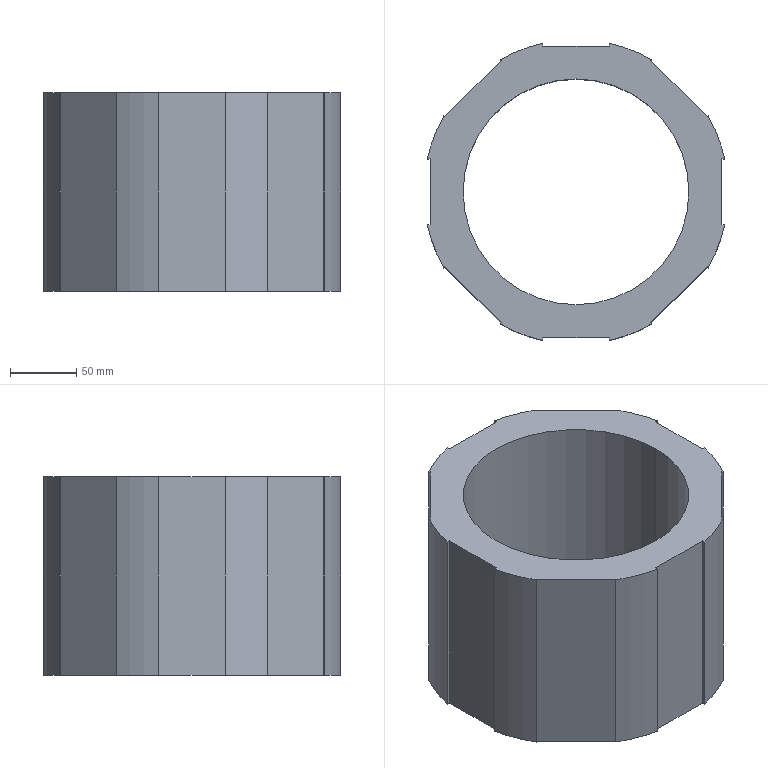Part | SolidWorks | features BaseBody 1 | 1 solid | 36 faces | box 224.499 x 224.499 x 150 mm | volume 2556210 mm3 | plane 26 | cylinder 10 | commonest cylinder face diameters 230 x8 170.4 x2
STEP:
#1=CARTESIAN_POINT('',(3283.116,1353.372,150.));
#2=VERTEX_POINT('',#1);
#3=CARTESIAN_POINT('',(3453.516,1353.372,150.));
#4=VERTEX_POINT('',#3);
#5=CARTESIAN_POINT('',(3368.316,1353.372,150.));
#6=DIRECTION('',(0.,0.,1.));
#7=DIRECTION('',(1.,0.,0.));
#8=AXIS2_PLACEMENT_3D('',#5,#6,#7);
#9=CIRCLE('',#8,85.2);
#10=EDGE_CURVE('',#2,#4,#9,.T.);
#11=ORIENTED_EDGE('',*,*,#10,.T.);
#12=CARTESIAN_POINT('',(3453.516,1353.372,0.));
#13=VERTEX_POINT('',#12);
#14=CARTESIAN_POINT('',(3453.516,1353.372,150.));
#15=DIRECTION('',(0.,0.,-1.));
#16=VECTOR('',#15,1000.);
#17=LINE('',#14,#16);
#18=EDGE_CURVE('',#4,#13,#17,.T.);
#19=ORIENTED_EDGE('',*,*,#18,.T.);
#20=CARTESIAN_POINT('',(3283.116,1353.372,0.));
#21=VERTEX_POINT('',#20);
#22=CARTESIAN_POINT('',(3368.316,1353.372,0.));
#23=DIRECTION('',(0.,0.,1.));
#24=DIRECTION('',(1.,0.,0.));
#25=AXIS2_PLACEMENT_3D('',#22,#23,#24);
#26=CIRCLE('',#25,85.2);
#27=EDGE_CURVE('',#21,#13,#26,.T.);
#28=ORIENTED_EDGE('',*,*,#27,.F.);
#29=CARTESIAN_POINT('',(3283.116,1353.372,150.));
#30=DIRECTION('',(0.,0.,-1.));
#31=VECTOR('',#30,1000.);
#32=LINE('',#29,#31);
#33=EDGE_CURVE('',#2,#21,#32,.T.);
#34=ORIENTED_EDGE('',*,*,#33,.F.);
#35=EDGE_LOOP('',(#11,#19,#28,#34));
#36=FACE_OUTER_BOUND('',#35,.T.);
#37=CARTESIAN_POINT('',(3368.316,1353.372,150.));
#38=DIRECTION('',(0.,0.,-1.));
#39=DIRECTION('',(-1.,0.,0.));
#40=AXIS2_PLACEMENT_3D('',#37,#38,#39);
#41=CYLINDRICAL_SURFACE('',#40,85.2);
#42=ADVANCED_FACE('',(#36),#41,.F.);
#43=CARTESIAN_POINT('',(3425.604,1453.087,150.));
#44=VERTEX_POINT('',#43);
#45=CARTESIAN_POINT('',(3393.316,1465.622,150.));
#46=VERTEX_POINT('',#45);
#47=CARTESIAN_POINT('',(3368.316,1353.372,150.));
#48=DIRECTION('',(0.,0.,1.));
#49=DIRECTION('',(1.,0.,0.));
#50=AXIS2_PLACEMENT_3D('',#47,#48,#49);
#51=CIRCLE('',#50,115.);
#52=EDGE_CURVE('',#44,#46,#51,.T.);
#53=ORIENTED_EDGE('',*,*,#52,.T.);
#54=CARTESIAN_POINT('',(3393.316,1463.372,150.));
#55=VERTEX_POINT('',#54);
#56=CARTESIAN_POINT('',(3393.316,1465.622,150.));
#57=DIRECTION('',(0.,-1.,0.));
#58=VECTOR('',#57,1000.);
#59=LINE('',#56,#58);
#60=EDGE_CURVE('',#46,#55,#59,.T.);
#61=ORIENTED_EDGE('',*,*,#60,.T.);
#62=CARTESIAN_POINT('',(3343.316,1463.372,150.));
#63=VERTEX_POINT('',#62);
#64=CARTESIAN_POINT('',(3393.316,1463.372,150.));
#65=DIRECTION('',(-1.,0.,0.));
#66=VECTOR('',#65,1000.);
#67=LINE('',#64,#66);
#68=EDGE_CURVE('',#55,#63,#67,.T.);
#69=ORIENTED_EDGE('',*,*,#68,.T.);
#70=CARTESIAN_POINT('',(3343.316,1465.622,150.));
#71=VERTEX_POINT('',#70);
#72=CARTESIAN_POINT('',(3343.316,1463.372,150.));
#73=DIRECTION('',(0.,1.,0.));
#74=VECTOR('',#73,1000.);
#75=LINE('',#72,#74);
#76=EDGE_CURVE('',#63,#71,#75,.T.);
#77=ORIENTED_EDGE('',*,*,#76,.T.);
#78=CARTESIAN_POINT('',(3311.028,1453.087,150.));
#79=VERTEX_POINT('',#78);
#80=CARTESIAN_POINT('',(3368.316,1353.372,150.));
#81=DIRECTION('',(0.,0.,1.));
#82=DIRECTION('',(1.,0.,0.));
#83=AXIS2_PLACEMENT_3D('',#80,#81,#82);
#84=CIRCLE('',#83,115.);
#85=EDGE_CURVE('',#71,#79,#84,.T.);
#86=ORIENTED_EDGE('',*,*,#85,.T.);
#87=CARTESIAN_POINT('',(3311.747,1452.367,150.));
#88=VERTEX_POINT('',#87);
#89=CARTESIAN_POINT('',(3311.028,1453.087,150.));
#90=DIRECTION('',(0.7071,-0.7071,0.));
#91=VECTOR('',#90,1000.);
#92=LINE('',#89,#91);
#93=EDGE_CURVE('',#79,#88,#92,.T.);
#94=ORIENTED_EDGE('',*,*,#93,.T.);
#95=CARTESIAN_POINT('',(3269.321,1409.941,150.));
#96=VERTEX_POINT('',#95);
#97=CARTESIAN_POINT('',(3311.747,1452.367,150.));
#98=DIRECTION('',(-0.7071,-0.7071,0.));
#99=VECTOR('',#98,1000.);
#100=LINE('',#97,#99);
#101=EDGE_CURVE('',#88,#96,#100,.T.);
#102=ORIENTED_EDGE('',*,*,#101,.T.);
#103=CARTESIAN_POINT('',(3268.601,1410.661,150.));
#104=VERTEX_POINT('',#103);
#105=CARTESIAN_POINT('',(3269.321,1409.941,150.));
#106=DIRECTION('',(-0.7071,0.7071,0.));
#107=VECTOR('',#106,1000.);
#108=LINE('',#105,#107);
#109=EDGE_CURVE('',#96,#104,#108,.T.);
#110=ORIENTED_EDGE('',*,*,#109,.T.);
#111=CARTESIAN_POINT('',(3256.066,1378.372,150.));
#112=VERTEX_POINT('',#111);
#113=CARTESIAN_POINT('',(3368.316,1353.372,150.));
#114=DIRECTION('',(0.,0.,1.));
#115=DIRECTION('',(1.,0.,0.));
#116=AXIS2_PLACEMENT_3D('',#113,#114,#115);
#117=CIRCLE('',#116,115.);
#118=EDGE_CURVE('',#104,#112,#117,.T.);
#119=ORIENTED_EDGE('',*,*,#118,.T.);
#120=CARTESIAN_POINT('',(3258.316,1378.372,150.));
#121=VERTEX_POINT('',#120);
#122=CARTESIAN_POINT('',(3256.066,1378.372,150.));
#123=DIRECTION('',(1.,0.,0.));
#124=VECTOR('',#123,1000.);
#125=LINE('',#122,#124);
#126=EDGE_CURVE('',#112,#121,#125,.T.);
#127=ORIENTED_EDGE('',*,*,#126,.T.);
#128=CARTESIAN_POINT('',(3258.316,1328.372,150.));
#129=VERTEX_POINT('',#128);
#130=CARTESIAN_POINT('',(3258.316,1378.372,150.));
#131=DIRECTION('',(0.,-1.,0.));
#132=VECTOR('',#131,1000.);
#133=LINE('',#130,#132);
#134=EDGE_CURVE('',#121,#129,#133,.T.);
#135=ORIENTED_EDGE('',*,*,#134,.T.);
#136=CARTESIAN_POINT('',(3256.066,1328.372,150.));
#137=VERTEX_POINT('',#136);
#138=CARTESIAN_POINT('',(3258.316,1328.372,150.));
#139=DIRECTION('',(-1.,0.,0.));
#140=VECTOR('',#139,1000.);
#141=LINE('',#138,#140);
#142=EDGE_CURVE('',#129,#137,#141,.T.);
#143=ORIENTED_EDGE('',*,*,#142,.T.);
#144=CARTESIAN_POINT('',(3268.601,1296.084,150.));
#145=VERTEX_POINT('',#144);
#146=CARTESIAN_POINT('',(3368.316,1353.372,150.));
#147=DIRECTION('',(0.,0.,1.));
#148=DIRECTION('',(1.,0.,0.));
#149=AXIS2_PLACEMENT_3D('',#146,#147,#148);
#150=CIRCLE('',#149,115.);
#151=EDGE_CURVE('',#137,#145,#150,.T.);
#152=ORIENTED_EDGE('',*,*,#151,.T.);
#153=CARTESIAN_POINT('',(3269.321,1296.804,150.));
#154=VERTEX_POINT('',#153);
#155=CARTESIAN_POINT('',(3268.601,1296.084,150.));
#156=DIRECTION('',(0.7071,0.7071,0.));
#157=VECTOR('',#156,1000.);
#158=LINE('',#155,#157);
#159=EDGE_CURVE('',#145,#154,#158,.T.);
#160=ORIENTED_EDGE('',*,*,#159,.T.);
#161=CARTESIAN_POINT('',(3311.747,1254.377,150.));
#162=VERTEX_POINT('',#161);
#163=CARTESIAN_POINT('',(3269.321,1296.804,150.));
#164=DIRECTION('',(0.7071,-0.7071,0.));
#165=VECTOR('',#164,1000.);
#166=LINE('',#163,#165);
#167=EDGE_CURVE('',#154,#162,#166,.T.);
#168=ORIENTED_EDGE('',*,*,#167,.T.);
#169=CARTESIAN_POINT('',(3311.028,1253.658,150.));
#170=VERTEX_POINT('',#169);
#171=CARTESIAN_POINT('',(3311.747,1254.377,150.));
#172=DIRECTION('',(-0.7071,-0.7071,0.));
#173=VECTOR('',#172,1000.);
#174=LINE('',#171,#173);
#175=EDGE_CURVE('',#162,#170,#174,.T.);
#176=ORIENTED_EDGE('',*,*,#175,.T.);
#177=CARTESIAN_POINT('',(3343.316,1241.123,150.));
#178=VERTEX_POINT('',#177);
#179=CARTESIAN_POINT('',(3368.316,1353.372,150.));
#180=DIRECTION('',(0.,0.,1.));
#181=DIRECTION('',(1.,0.,0.));
#182=AXIS2_PLACEMENT_3D('',#179,#180,#181);
#183=CIRCLE('',#182,115.);
#184=EDGE_CURVE('',#170,#178,#183,.T.);
#185=ORIENTED_EDGE('',*,*,#184,.T.);
#186=CARTESIAN_POINT('',(3343.316,1243.372,150.));
#187=VERTEX_POINT('',#186);
#188=CARTESIAN_POINT('',(3343.316,1241.123,150.));
#189=DIRECTION('',(0.,1.,0.));
#190=VECTOR('',#189,1000.);
#191=LINE('',#188,#190);
#192=EDGE_CURVE('',#178,#187,#191,.T.);
#193=ORIENTED_EDGE('',*,*,#192,.T.);
#194=CARTESIAN_POINT('',(3393.316,1243.372,150.));
#195=VERTEX_POINT('',#194);
#196=CARTESIAN_POINT('',(3343.316,1243.372,150.));
#197=DIRECTION('',(1.,0.,0.));
#198=VECTOR('',#197,1000.);
#199=LINE('',#196,#198);
#200=EDGE_CURVE('',#187,#195,#199,.T.);
#201=ORIENTED_EDGE('',*,*,#200,.T.);
#202=CARTESIAN_POINT('',(3393.316,1241.123,150.));
#203=VERTEX_POINT('',#202);
#204=CARTESIAN_POINT('',(3393.316,1243.372,150.));
#205=DIRECTION('',(0.,-1.,0.));
#206=VECTOR('',#205,1000.);
#207=LINE('',#204,#206);
#208=EDGE_CURVE('',#195,#203,#207,.T.);
#209=ORIENTED_EDGE('',*,*,#208,.T.);
#210=CARTESIAN_POINT('',(3425.604,1253.658,150.));
#211=VERTEX_POINT('',#210);
#212=CARTESIAN_POINT('',(3368.316,1353.372,150.));
#213=DIRECTION('',(0.,0.,1.));
#214=DIRECTION('',(1.,0.,0.));
#215=AXIS2_PLACEMENT_3D('',#212,#213,#214);
#216=CIRCLE('',#215,115.);
#217=EDGE_CURVE('',#203,#211,#216,.T.);
#218=ORIENTED_EDGE('',*,*,#217,.T.);
#219=CARTESIAN_POINT('',(3424.884,1254.377,150.));
#220=VERTEX_POINT('',#219);
#221=CARTESIAN_POINT('',(3425.604,1253.658,150.));
#222=DIRECTION('',(-0.7071,0.7071,0.));
#223=VECTOR('',#222,1000.);
#224=LINE('',#221,#223);
#225=EDGE_CURVE('',#211,#220,#224,.T.);
#226=ORIENTED_EDGE('',*,*,#225,.T.);
#227=CARTESIAN_POINT('',(3467.311,1296.804,150.));
#228=VERTEX_POINT('',#227);
#229=CARTESIAN_POINT('',(3424.884,1254.377,150.));
#230=DIRECTION('',(0.7071,0.7071,0.));
#231=VECTOR('',#230,1000.);
#232=LINE('',#229,#231);
#233=EDGE_CURVE('',#220,#228,#232,.T.);
#234=ORIENTED_EDGE('',*,*,#233,.T.);
#235=CARTESIAN_POINT('',(3468.031,1296.084,150.));
#236=VERTEX_POINT('',#235);
#237=CARTESIAN_POINT('',(3467.311,1296.804,150.));
#238=DIRECTION('',(0.7071,-0.7071,0.));
#239=VECTOR('',#238,1000.);
#240=LINE('',#237,#239);
#241=EDGE_CURVE('',#228,#236,#240,.T.);
#242=ORIENTED_EDGE('',*,*,#241,.T.);
#243=CARTESIAN_POINT('',(3480.566,1328.372,150.));
#244=VERTEX_POINT('',#243);
#245=CARTESIAN_POINT('',(3368.316,1353.372,150.));
#246=DIRECTION('',(0.,0.,1.));
#247=DIRECTION('',(1.,0.,0.));
#248=AXIS2_PLACEMENT_3D('',#245,#246,#247);
#249=CIRCLE('',#248,115.);
#250=EDGE_CURVE('',#236,#244,#249,.T.);
#251=ORIENTED_EDGE('',*,*,#250,.T.);
#252=CARTESIAN_POINT('',(3478.316,1328.372,150.));
#253=VERTEX_POINT('',#252);
#254=CARTESIAN_POINT('',(3480.566,1328.372,150.));
#255=DIRECTION('',(-1.,0.,0.));
#256=VECTOR('',#255,1000.);
#257=LINE('',#254,#256);
#258=EDGE_CURVE('',#244,#253,#257,.T.);
#259=ORIENTED_EDGE('',*,*,#258,.T.);
#260=CARTESIAN_POINT('',(3478.316,1378.372,150.));
#261=VERTEX_POINT('',#260);
#262=CARTESIAN_POINT('',(3478.316,1328.372,150.));
#263=DIRECTION('',(0.,1.,0.));
#264=VECTOR('',#263,1000.);
#265=LINE('',#262,#264);
#266=EDGE_CURVE('',#253,#261,#265,.T.);
#267=ORIENTED_EDGE('',*,*,#266,.T.);
#268=CARTESIAN_POINT('',(3480.566,1378.372,150.));
#269=VERTEX_POINT('',#268);
#270=CARTESIAN_POINT('',(3478.316,1378.372,150.));
#271=DIRECTION('',(1.,0.,0.));
#272=VECTOR('',#271,1000.);
#273=LINE('',#270,#272);
#274=EDGE_CURVE('',#261,#269,#273,.T.);
#275=ORIENTED_EDGE('',*,*,#274,.T.);
#276=CARTESIAN_POINT('',(3468.031,1410.661,150.));
#277=VERTEX_POINT('',#276);
#278=CARTESIAN_POINT('',(3368.316,1353.372,150.));
#279=DIRECTION('',(0.,0.,1.));
#280=DIRECTION('',(1.,0.,0.));
#281=AXIS2_PLACEMENT_3D('',#278,#279,#280);
#282=CIRCLE('',#281,115.);
#283=EDGE_CURVE('',#269,#277,#282,.T.);
#284=ORIENTED_EDGE('',*,*,#283,.T.);
#285=CARTESIAN_POINT('',(3467.311,1409.941,150.));
#286=VERTEX_POINT('',#285);
#287=CARTESIAN_POINT('',(3468.031,1410.661,150.));
#288=DIRECTION('',(-0.7071,-0.7071,0.));
#289=VECTOR('',#288,1000.);
#290=LINE('',#287,#289);
#291=EDGE_CURVE('',#277,#286,#290,.T.);
#292=ORIENTED_EDGE('',*,*,#291,.T.);
#293=CARTESIAN_POINT('',(3424.884,1452.367,150.));
#294=VERTEX_POINT('',#293);
#295=CARTESIAN_POINT('',(3467.311,1409.941,150.));
#296=DIRECTION('',(-0.7071,0.7071,0.));
#297=VECTOR('',#296,1000.);
#298=LINE('',#295,#297);
#299=EDGE_CURVE('',#286,#294,#298,.T.);
#300=ORIENTED_EDGE('',*,*,#299,.T.);
#301=CARTESIAN_POINT('',(3424.884,1452.367,150.));
#302=DIRECTION('',(0.7071,0.7071,0.));
#303=VECTOR('',#302,1000.);
#304=LINE('',#301,#303);
#305=EDGE_CURVE('',#294,#44,#304,.T.);
#306=ORIENTED_EDGE('',*,*,#305,.T.);
#307=EDGE_LOOP('',(#53,#61,#69,#77,#86,#94,#102,#110,#119,#127,#135,#143,#152,#160,#168,#176,#185,#193,#201,#209,#218,#226,#234,#242,#251,#259,#267,#275,#284,#292,#300,#306));
#308=FACE_OUTER_BOUND('',#307,.T.);
#309=ORIENTED_EDGE('',*,*,#10,.F.);
#310=CARTESIAN_POINT('',(3368.316,1353.372,150.));
#311=DIRECTION('',(0.,0.,1.));
#312=DIRECTION('',(1.,0.,0.));
#313=AXIS2_PLACEMENT_3D('',#310,#311,#312);
#314=CIRCLE('',#313,85.2);
#315=EDGE_CURVE('',#4,#2,#314,.T.);
#316=ORIENTED_EDGE('',*,*,#315,.F.);
#317=EDGE_LOOP('',(#309,#316));
#318=FACE_BOUND('',#317,.T.);
#319=CARTESIAN_POINT('',(3368.316,1353.372,150.));
#320=DIRECTION('',(0.,0.,1.));
#321=DIRECTION('',(1.,0.,0.));
#322=AXIS2_PLACEMENT_3D('',#319,#320,#321);
#323=PLANE('',#322);
#324=ADVANCED_FACE('',(#308,#318),#323,.T.);
#325=CARTESIAN_POINT('',(3425.604,1453.087,0.));
#326=VERTEX_POINT('',#325);
#327=CARTESIAN_POINT('',(3393.316,1465.622,0.));
#328=VERTEX_POINT('',#327);
#329=CARTESIAN_POINT('',(3368.316,1353.372,0.));
#330=DIRECTION('',(0.,0.,1.));
#331=DIRECTION('',(1.,0.,0.));
#332=AXIS2_PLACEMENT_3D('',#329,#330,#331);
#333=CIRCLE('',#332,115.);
#334=EDGE_CURVE('',#326,#328,#333,.T.);
#335=ORIENTED_EDGE('',*,*,#334,.F.);
#336=CARTESIAN_POINT('',(3424.884,1452.367,0.));
#337=VERTEX_POINT('',#336);
#338=CARTESIAN_POINT('',(3424.884,1452.367,0.));
#339=DIRECTION('',(0.7071,0.7071,0.));
#340=VECTOR('',#339,1000.);
#341=LINE('',#338,#340);
#342=EDGE_CURVE('',#337,#326,#341,.T.);
#343=ORIENTED_EDGE('',*,*,#342,.F.);
#344=CARTESIAN_POINT('',(3467.311,1409.941,0.));
#345=VERTEX_POINT('',#344);
#346=CARTESIAN_POINT('',(3467.311,1409.941,0.));
#347=DIRECTION('',(-0.7071,0.7071,0.));
#348=VECTOR('',#347,1000.);
#349=LINE('',#346,#348);
#350=EDGE_CURVE('',#345,#337,#349,.T.);
#351=ORIENTED_EDGE('',*,*,#350,.F.);
#352=CARTESIAN_POINT('',(3468.031,1410.661,0.));
#353=VERTEX_POINT('',#352);
#354=CARTESIAN_POINT('',(3468.031,1410.661,0.));
#355=DIRECTION('',(-0.7071,-0.7071,0.));
#356=VECTOR('',#355,1000.);
#357=LINE('',#354,#356);
#358=EDGE_CURVE('',#353,#345,#357,.T.);
#359=ORIENTED_EDGE('',*,*,#358,.F.);
#360=CARTESIAN_POINT('',(3480.566,1378.372,0.));
#361=VERTEX_POINT('',#360);
#362=CARTESIAN_POINT('',(3368.316,1353.372,0.));
#363=DIRECTION('',(0.,0.,1.));
#364=DIRECTION('',(1.,0.,0.));
#365=AXIS2_PLACEMENT_3D('',#362,#363,#364);
#366=CIRCLE('',#365,115.);
#367=EDGE_CURVE('',#361,#353,#366,.T.);
#368=ORIENTED_EDGE('',*,*,#367,.F.);
#369=CARTESIAN_POINT('',(3478.316,1378.372,0.));
#370=VERTEX_POINT('',#369);
#371=CARTESIAN_POINT('',(3478.316,1378.372,0.));
#372=DIRECTION('',(1.,0.,0.));
#373=VECTOR('',#372,1000.);
#374=LINE('',#371,#373);
#375=EDGE_CURVE('',#370,#361,#374,.T.);
#376=ORIENTED_EDGE('',*,*,#375,.F.);
#377=CARTESIAN_POINT('',(3478.316,1328.372,0.));
#378=VERTEX_POINT('',#377);
#379=CARTESIAN_POINT('',(3478.316,1328.372,0.));
#380=DIRECTION('',(0.,1.,0.));
#381=VECTOR('',#380,1000.);
#382=LINE('',#379,#381);
#383=EDGE_CURVE('',#378,#370,#382,.T.);
#384=ORIENTED_EDGE('',*,*,#383,.F.);
#385=CARTESIAN_POINT('',(3480.566,1328.372,0.));
#386=VERTEX_POINT('',#385);
#387=CARTESIAN_POINT('',(3480.566,1328.372,0.));
#388=DIRECTION('',(-1.,0.,0.));
#389=VECTOR('',#388,1000.);
#390=LINE('',#387,#389);
#391=EDGE_CURVE('',#386,#378,#390,.T.);
#392=ORIENTED_EDGE('',*,*,#391,.F.);
#393=CARTESIAN_POINT('',(3468.031,1296.084,0.));
#394=VERTEX_POINT('',#393);
#395=CARTESIAN_POINT('',(3368.316,1353.372,0.));
#396=DIRECTION('',(0.,0.,1.));
#397=DIRECTION('',(1.,0.,0.));
#398=AXIS2_PLACEMENT_3D('',#395,#396,#397);
#399=CIRCLE('',#398,115.);
#400=EDGE_CURVE('',#394,#386,#399,.T.);
#401=ORIENTED_EDGE('',*,*,#400,.F.);
#402=CARTESIAN_POINT('',(3467.311,1296.804,0.));
#403=VERTEX_POINT('',#402);
#404=CARTESIAN_POINT('',(3467.311,1296.804,0.));
#405=DIRECTION('',(0.7071,-0.7071,0.));
#406=VECTOR('',#405,1000.);
#407=LINE('',#404,#406);
#408=EDGE_CURVE('',#403,#394,#407,.T.);
#409=ORIENTED_EDGE('',*,*,#408,.F.);
#410=CARTESIAN_POINT('',(3424.884,1254.377,0.));
#411=VERTEX_POINT('',#410);
#412=CARTESIAN_POINT('',(3424.884,1254.377,0.));
#413=DIRECTION('',(0.7071,0.7071,0.));
#414=VECTOR('',#413,1000.);
#415=LINE('',#412,#414);
#416=EDGE_CURVE('',#411,#403,#415,.T.);
#417=ORIENTED_EDGE('',*,*,#416,.F.);
#418=CARTESIAN_POINT('',(3425.604,1253.658,0.));
#419=VERTEX_POINT('',#418);
#420=CARTESIAN_POINT('',(3425.604,1253.658,0.));
#421=DIRECTION('',(-0.7071,0.7071,0.));
#422=VECTOR('',#421,1000.);
#423=LINE('',#420,#422);
#424=EDGE_CURVE('',#419,#411,#423,.T.);
#425=ORIENTED_EDGE('',*,*,#424,.F.);
#426=CARTESIAN_POINT('',(3393.316,1241.123,0.));
#427=VERTEX_POINT('',#426);
#428=CARTESIAN_POINT('',(3368.316,1353.372,0.));
#429=DIRECTION('',(0.,0.,1.));
#430=DIRECTION('',(1.,0.,0.));
#431=AXIS2_PLACEMENT_3D('',#428,#429,#430);
#432=CIRCLE('',#431,115.);
#433=EDGE_CURVE('',#427,#419,#432,.T.);
#434=ORIENTED_EDGE('',*,*,#433,.F.);
#435=CARTESIAN_POINT('',(3393.316,1243.372,0.));
#436=VERTEX_POINT('',#435);
#437=CARTESIAN_POINT('',(3393.316,1243.372,0.));
#438=DIRECTION('',(0.,-1.,0.));
#439=VECTOR('',#438,1000.);
#440=LINE('',#437,#439);
#441=EDGE_CURVE('',#436,#427,#440,.T.);
#442=ORIENTED_EDGE('',*,*,#441,.F.);
#443=CARTESIAN_POINT('',(3343.316,1243.372,0.));
#444=VERTEX_POINT('',#443);
#445=CARTESIAN_POINT('',(3343.316,1243.372,0.));
#446=DIRECTION('',(1.,0.,0.));
#447=VECTOR('',#446,1000.);
#448=LINE('',#445,#447);
#449=EDGE_CURVE('',#444,#436,#448,.T.);
#450=ORIENTED_EDGE('',*,*,#449,.F.);
#451=CARTESIAN_POINT('',(3343.316,1241.123,0.));
#452=VERTEX_POINT('',#451);
#453=CARTESIAN_POINT('',(3343.316,1241.123,0.));
#454=DIRECTION('',(0.,1.,0.));
#455=VECTOR('',#454,1000.);
#456=LINE('',#453,#455);
#457=EDGE_CURVE('',#452,#444,#456,.T.);
#458=ORIENTED_EDGE('',*,*,#457,.F.);
#459=CARTESIAN_POINT('',(3311.028,1253.658,0.));
#460=VERTEX_POINT('',#459);
#461=CARTESIAN_POINT('',(3368.316,1353.372,0.));
#462=DIRECTION('',(0.,0.,1.));
#463=DIRECTION('',(1.,0.,0.));
#464=AXIS2_PLACEMENT_3D('',#461,#462,#463);
#465=CIRCLE('',#464,115.);
#466=EDGE_CURVE('',#460,#452,#465,.T.);
#467=ORIENTED_EDGE('',*,*,#466,.F.);
#468=CARTESIAN_POINT('',(3311.747,1254.377,0.));
#469=VERTEX_POINT('',#468);
#470=CARTESIAN_POINT('',(3311.747,1254.377,0.));
#471=DIRECTION('',(-0.7071,-0.7071,0.));
#472=VECTOR('',#471,1000.);
#473=LINE('',#470,#472);
#474=EDGE_CURVE('',#469,#460,#473,.T.);
#475=ORIENTED_EDGE('',*,*,#474,.F.);
#476=CARTESIAN_POINT('',(3269.321,1296.804,0.));
#477=VERTEX_POINT('',#476);
#478=CARTESIAN_POINT('',(3269.321,1296.804,0.));
#479=DIRECTION('',(0.7071,-0.7071,0.));
#480=VECTOR('',#479,1000.);
#481=LINE('',#478,#480);
#482=EDGE_CURVE('',#477,#469,#481,.T.);
#483=ORIENTED_EDGE('',*,*,#482,.F.);
#484=CARTESIAN_POINT('',(3268.601,1296.084,0.));
#485=VERTEX_POINT('',#484);
#486=CARTESIAN_POINT('',(3268.601,1296.084,0.));
#487=DIRECTION('',(0.7071,0.7071,0.));
#488=VECTOR('',#487,1000.);
#489=LINE('',#486,#488);
#490=EDGE_CURVE('',#485,#477,#489,.T.);
#491=ORIENTED_EDGE('',*,*,#490,.F.);
#492=CARTESIAN_POINT('',(3256.066,1328.372,0.));
#493=VERTEX_POINT('',#492);
#494=CARTESIAN_POINT('',(3368.316,1353.372,0.));
#495=DIRECTION('',(0.,0.,1.));
#496=DIRECTION('',(1.,0.,0.));
#497=AXIS2_PLACEMENT_3D('',#494,#495,#496);
#498=CIRCLE('',#497,115.);
#499=EDGE_CURVE('',#493,#485,#498,.T.);
#500=ORIENTED_EDGE('',*,*,#499,.F.);
#501=CARTESIAN_POINT('',(3258.316,1328.372,0.));
#502=VERTEX_POINT('',#501);
#503=CARTESIAN_POINT('',(3258.316,1328.372,0.));
#504=DIRECTION('',(-1.,0.,0.));
#505=VECTOR('',#504,1000.);
#506=LINE('',#503,#505);
#507=EDGE_CURVE('',#502,#493,#506,.T.);
#508=ORIENTED_EDGE('',*,*,#507,.F.);
#509=CARTESIAN_POINT('',(3258.316,1378.372,0.));
#510=VERTEX_POINT('',#509);
#511=CARTESIAN_POINT('',(3258.316,1378.372,0.));
#512=DIRECTION('',(0.,-1.,0.));
#513=VECTOR('',#512,1000.);
#514=LINE('',#511,#513);
#515=EDGE_CURVE('',#510,#502,#514,.T.);
#516=ORIENTED_EDGE('',*,*,#515,.F.);
#517=CARTESIAN_POINT('',(3256.066,1378.372,0.));
#518=VERTEX_POINT('',#517);
#519=CARTESIAN_POINT('',(3256.066,1378.372,0.));
#520=DIRECTION('',(1.,0.,0.));
#521=VECTOR('',#520,1000.);
#522=LINE('',#519,#521);
#523=EDGE_CURVE('',#518,#510,#522,.T.);
#524=ORIENTED_EDGE('',*,*,#523,.F.);
#525=CARTESIAN_POINT('',(3268.601,1410.661,0.));
#526=VERTEX_POINT('',#525);
#527=CARTESIAN_POINT('',(3368.316,1353.372,0.));
#528=DIRECTION('',(0.,0.,1.));
#529=DIRECTION('',(1.,0.,0.));
#530=AXIS2_PLACEMENT_3D('',#527,#528,#529);
#531=CIRCLE('',#530,115.);
#532=EDGE_CURVE('',#526,#518,#531,.T.);
#533=ORIENTED_EDGE('',*,*,#532,.F.);
#534=CARTESIAN_POINT('',(3269.321,1409.941,0.));
#535=VERTEX_POINT('',#534);
#536=CARTESIAN_POINT('',(3269.321,1409.941,0.));
#537=DIRECTION('',(-0.7071,0.7071,0.));
#538=VECTOR('',#537,1000.);
#539=LINE('',#536,#538);
#540=EDGE_CURVE('',#535,#526,#539,.T.);
#541=ORIENTED_EDGE('',*,*,#540,.F.);
#542=CARTESIAN_POINT('',(3311.747,1452.367,0.));
#543=VERTEX_POINT('',#542);
#544=CARTESIAN_POINT('',(3311.747,1452.367,0.));
#545=DIRECTION('',(-0.7071,-0.7071,0.));
#546=VECTOR('',#545,1000.);
#547=LINE('',#544,#546);
#548=EDGE_CURVE('',#543,#535,#547,.T.);
#549=ORIENTED_EDGE('',*,*,#548,.F.);
#550=CARTESIAN_POINT('',(3311.028,1453.087,0.));
#551=VERTEX_POINT('',#550);
#552=CARTESIAN_POINT('',(3311.028,1453.087,0.));
#553=DIRECTION('',(0.7071,-0.7071,0.));
#554=VECTOR('',#553,1000.);
#555=LINE('',#552,#554);
#556=EDGE_CURVE('',#551,#543,#555,.T.);
#557=ORIENTED_EDGE('',*,*,#556,.F.);
#558=CARTESIAN_POINT('',(3343.316,1465.622,0.));
#559=VERTEX_POINT('',#558);
#560=CARTESIAN_POINT('',(3368.316,1353.372,0.));
#561=DIRECTION('',(0.,0.,1.));
#562=DIRECTION('',(1.,0.,0.));
#563=AXIS2_PLACEMENT_3D('',#560,#561,#562);
#564=CIRCLE('',#563,115.);
#565=EDGE_CURVE('',#559,#551,#564,.T.);
#566=ORIENTED_EDGE('',*,*,#565,.F.);
#567=CARTESIAN_POINT('',(3343.316,1463.372,0.));
#568=VERTEX_POINT('',#567);
#569=CARTESIAN_POINT('',(3343.316,1463.372,0.));
#570=DIRECTION('',(0.,1.,0.));
#571=VECTOR('',#570,1000.);
#572=LINE('',#569,#571);
#573=EDGE_CURVE('',#568,#559,#572,.T.);
#574=ORIENTED_EDGE('',*,*,#573,.F.);
#575=CARTESIAN_POINT('',(3393.316,1463.372,0.));
#576=VERTEX_POINT('',#575);
#577=CARTESIAN_POINT('',(3393.316,1463.372,0.));
#578=DIRECTION('',(-1.,0.,0.));
#579=VECTOR('',#578,1000.);
#580=LINE('',#577,#579);
#581=EDGE_CURVE('',#576,#568,#580,.T.);
#582=ORIENTED_EDGE('',*,*,#581,.F.);
#583=CARTESIAN_POINT('',(3393.316,1465.622,0.));
#584=DIRECTION('',(0.,-1.,0.));
#585=VECTOR('',#584,1000.);
#586=LINE('',#583,#585);
#587=EDGE_CURVE('',#328,#576,#586,.T.);
#588=ORIENTED_EDGE('',*,*,#587,.F.);
#589=EDGE_LOOP('',(#335,#343,#351,#359,#368,#376,#384,#392,#401,#409,#417,#425,#434,#442,#450,#458,#467,#475,#483,#491,#500,#508,#516,#524,#533,#541,#549,#557,#566,#574,#582,#588));
#590=FACE_OUTER_BOUND('',#589,.T.);
#591=ORIENTED_EDGE('',*,*,#27,.T.);
#592=CARTESIAN_POINT('',(3368.316,1353.372,0.));
#593=DIRECTION('',(0.,0.,1.));
#594=DIRECTION('',(1.,0.,0.));
#595=AXIS2_PLACEMENT_3D('',#592,#593,#594);
#596=CIRCLE('',#595,85.2);
#597=EDGE_CURVE('',#13,#21,#596,.T.);
#598=ORIENTED_EDGE('',*,*,#597,.T.);
#599=EDGE_LOOP('',(#591,#598));
#600=FACE_BOUND('',#599,.T.);
#601=CARTESIAN_POINT('',(3368.316,1353.372,0.));
#602=DIRECTION('',(0.,0.,1.));
#603=DIRECTION('',(1.,0.,0.));
#604=AXIS2_PLACEMENT_3D('',#601,#602,#603);
#605=PLANE('',#604);
#606=ADVANCED_FACE('',(#590,#600),#605,.F.);
#607=ORIENTED_EDGE('',*,*,#334,.T.);
#608=CARTESIAN_POINT('',(3393.316,1465.622,150.));
#609=DIRECTION('',(0.,0.,-1.));
#610=VECTOR('',#609,1000.);
#611=LINE('',#608,#610);
#612=EDGE_CURVE('',#46,#328,#611,.T.);
#613=ORIENTED_EDGE('',*,*,#612,.F.);
#614=ORIENTED_EDGE('',*,*,#52,.F.);
#615=CARTESIAN_POINT('',(3425.604,1453.087,150.));
#616=DIRECTION('',(0.,0.,-1.));
#617=VECTOR('',#616,1000.);
#618=LINE('',#615,#617);
#619=EDGE_CURVE('',#44,#326,#618,.T.);
#620=ORIENTED_EDGE('',*,*,#619,.T.);
#621=EDGE_LOOP('',(#607,#613,#614,#620));
#622=FACE_OUTER_BOUND('',#621,.T.);
#623=CARTESIAN_POINT('',(3368.316,1353.372,150.));
#624=DIRECTION('',(0.,0.,-1.));
#625=DIRECTION('',(-1.,0.,0.));
#626=AXIS2_PLACEMENT_3D('',#623,#624,#625);
#627=CYLINDRICAL_SURFACE('',#626,115.);
#628=ADVANCED_FACE('',(#622),#627,.T.);
#629=ORIENTED_EDGE('',*,*,#587,.T.);
#630=CARTESIAN_POINT('',(3393.316,1463.372,150.));
#631=DIRECTION('',(0.,0.,-1.));
#632=VECTOR('',#631,1000.);
#633=LINE('',#630,#632);
#634=EDGE_CURVE('',#55,#576,#633,.T.);
#635=ORIENTED_EDGE('',*,*,#634,.F.);
#636=ORIENTED_EDGE('',*,*,#60,.F.);
#637=ORIENTED_EDGE('',*,*,#612,.T.);
#638=EDGE_LOOP('',(#629,#635,#636,#637));
#639=FACE_OUTER_BOUND('',#638,.T.);
#640=CARTESIAN_POINT('',(3393.316,1465.622,150.));
#641=DIRECTION('',(1.,0.,0.));
#642=DIRECTION('',(0.,0.,-1.));
#643=AXIS2_PLACEMENT_3D('',#640,#641,#642);
#644=PLANE('',#643);
#645=ADVANCED_FACE('',(#639),#644,.F.);
#646=ORIENTED_EDGE('',*,*,#581,.T.);
#647=CARTESIAN_POINT('',(3343.316,1463.372,150.));
#648=DIRECTION('',(0.,0.,-1.));
#649=VECTOR('',#648,1000.);
#650=LINE('',#647,#649);
#651=EDGE_CURVE('',#63,#568,#650,.T.);
#652=ORIENTED_EDGE('',*,*,#651,.F.);
#653=ORIENTED_EDGE('',*,*,#68,.F.);
#654=ORIENTED_EDGE('',*,*,#634,.T.);
#655=EDGE_LOOP('',(#646,#652,#653,#654));
#656=FACE_OUTER_BOUND('',#655,.T.);
#657=CARTESIAN_POINT('',(3393.316,1463.372,150.));
#658=DIRECTION('',(0.,-1.,0.));
#659=DIRECTION('',(0.,0.,-1.));
#660=AXIS2_PLACEMENT_3D('',#657,#658,#659);
#661=PLANE('',#660);
#662=ADVANCED_FACE('',(#656),#661,.F.);
#663=ORIENTED_EDGE('',*,*,#573,.T.);
#664=CARTESIAN_POINT('',(3343.316,1465.622,150.));
#665=DIRECTION('',(0.,0.,-1.));
#666=VECTOR('',#665,1000.);
#667=LINE('',#664,#666);
#668=EDGE_CURVE('',#71,#559,#667,.T.);
#669=ORIENTED_EDGE('',*,*,#668,.F.);
#670=ORIENTED_EDGE('',*,*,#76,.F.);
#671=ORIENTED_EDGE('',*,*,#651,.T.);
#672=EDGE_LOOP('',(#663,#669,#670,#671));
#673=FACE_OUTER_BOUND('',#672,.T.);
#674=CARTESIAN_POINT('',(3343.316,1463.372,150.));
#675=DIRECTION('',(-1.,0.,0.));
#676=DIRECTION('',(0.,0.,1.));
#677=AXIS2_PLACEMENT_3D('',#674,#675,#676);
#678=PLANE('',#677);
#679=ADVANCED_FACE('',(#673),#678,.F.);
#680=ORIENTED_EDGE('',*,*,#565,.T.);
#681=CARTESIAN_POINT('',(3311.028,1453.087,150.));
#682=DIRECTION('',(0.,0.,-1.));
#683=VECTOR('',#682,1000.);
#684=LINE('',#681,#683);
#685=EDGE_CURVE('',#79,#551,#684,.T.);
#686=ORIENTED_EDGE('',*,*,#685,.F.);
#687=ORIENTED_EDGE('',*,*,#85,.F.);
#688=ORIENTED_EDGE('',*,*,#668,.T.);
#689=EDGE_LOOP('',(#680,#686,#687,#688));
#690=FACE_OUTER_BOUND('',#689,.T.);
#691=CARTESIAN_POINT('',(3368.316,1353.372,150.));
#692=DIRECTION('',(0.,0.,-1.));
#693=DIRECTION('',(-1.,0.,0.));
#694=AXIS2_PLACEMENT_3D('',#691,#692,#693);
#695=CYLINDRICAL_SURFACE('',#694,115.);
#696=ADVANCED_FACE('',(#690),#695,.T.);
#697=ORIENTED_EDGE('',*,*,#556,.T.);
#698=CARTESIAN_POINT('',(3311.747,1452.367,150.));
#699=DIRECTION('',(0.,0.,-1.));
#700=VECTOR('',#699,1000.);
#701=LINE('',#698,#700);
#702=EDGE_CURVE('',#88,#543,#701,.T.);
#703=ORIENTED_EDGE('',*,*,#702,.F.);
#704=ORIENTED_EDGE('',*,*,#93,.F.);
#705=ORIENTED_EDGE('',*,*,#685,.T.);
#706=EDGE_LOOP('',(#697,#703,#704,#705));
#707=FACE_OUTER_BOUND('',#706,.T.);
#708=CARTESIAN_POINT('',(3311.028,1453.087,150.));
#709=DIRECTION('',(0.7071,0.7071,0.));
#710=DIRECTION('',(-0.7071,0.7071,0.));
#711=AXIS2_PLACEMENT_3D('',#708,#709,#710);
#712=PLANE('',#711);
#713=ADVANCED_FACE('',(#707),#712,.F.);
#714=ORIENTED_EDGE('',*,*,#548,.T.);
#715=CARTESIAN_POINT('',(3269.321,1409.941,150.));
#716=DIRECTION('',(0.,0.,-1.));
#717=VECTOR('',#716,1000.);
#718=LINE('',#715,#717);
#719=EDGE_CURVE('',#96,#535,#718,.T.);
#720=ORIENTED_EDGE('',*,*,#719,.F.);
#721=ORIENTED_EDGE('',*,*,#101,.F.);
#722=ORIENTED_EDGE('',*,*,#702,.T.);
#723=EDGE_LOOP('',(#714,#720,#721,#722));
#724=FACE_OUTER_BOUND('',#723,.T.);
#725=CARTESIAN_POINT('',(3311.747,1452.367,150.));
#726=DIRECTION('',(0.7071,-0.7071,0.));
#727=DIRECTION('',(0.7071,0.7071,0.));
#728=AXIS2_PLACEMENT_3D('',#725,#726,#727);
#729=PLANE('',#728);
#730=ADVANCED_FACE('',(#724),#729,.F.);
#731=ORIENTED_EDGE('',*,*,#540,.T.);
#732=CARTESIAN_POINT('',(3268.601,1410.661,150.));
#733=DIRECTION('',(0.,0.,-1.));
#734=VECTOR('',#733,1000.);
#735=LINE('',#732,#734);
#736=EDGE_CURVE('',#104,#526,#735,.T.);
#737=ORIENTED_EDGE('',*,*,#736,.F.);
#738=ORIENTED_EDGE('',*,*,#109,.F.);
#739=ORIENTED_EDGE('',*,*,#719,.T.);
#740=EDGE_LOOP('',(#731,#737,#738,#739));
#741=FACE_OUTER_BOUND('',#740,.T.);
#742=CARTESIAN_POINT('',(3269.321,1409.941,150.));
#743=DIRECTION('',(-0.7071,-0.7071,0.));
#744=DIRECTION('',(0.7071,-0.7071,0.));
#745=AXIS2_PLACEMENT_3D('',#742,#743,#744);
#746=PLANE('',#745);
#747=ADVANCED_FACE('',(#741),#746,.F.);
#748=ORIENTED_EDGE('',*,*,#532,.T.);
#749=CARTESIAN_POINT('',(3256.066,1378.372,150.));
#750=DIRECTION('',(0.,0.,-1.));
#751=VECTOR('',#750,1000.);
#752=LINE('',#749,#751);
#753=EDGE_CURVE('',#112,#518,#752,.T.);
#754=ORIENTED_EDGE('',*,*,#753,.F.);
#755=ORIENTED_EDGE('',*,*,#118,.F.);
#756=ORIENTED_EDGE('',*,*,#736,.T.);
#757=EDGE_LOOP('',(#748,#754,#755,#756));
#758=FACE_OUTER_BOUND('',#757,.T.);
#759=CARTESIAN_POINT('',(3368.316,1353.372,150.));
#760=DIRECTION('',(0.,0.,-1.));
#761=DIRECTION('',(-1.,0.,0.));
#762=AXIS2_PLACEMENT_3D('',#759,#760,#761);
#763=CYLINDRICAL_SURFACE('',#762,115.);
#764=ADVANCED_FACE('',(#758),#763,.T.);
#765=ORIENTED_EDGE('',*,*,#523,.T.);
#766=CARTESIAN_POINT('',(3258.316,1378.372,150.));
#767=DIRECTION('',(0.,0.,-1.));
#768=VECTOR('',#767,1000.);
#769=LINE('',#766,#768);
#770=EDGE_CURVE('',#121,#510,#769,.T.);
#771=ORIENTED_EDGE('',*,*,#770,.F.);
#772=ORIENTED_EDGE('',*,*,#126,.F.);
#773=ORIENTED_EDGE('',*,*,#753,.T.);
#774=EDGE_LOOP('',(#765,#771,#772,#773));
#775=FACE_OUTER_BOUND('',#774,.T.);
#776=CARTESIAN_POINT('',(3256.066,1378.372,150.));
#777=DIRECTION('',(0.,1.,0.));
#778=DIRECTION('',(0.,0.,1.));
#779=AXIS2_PLACEMENT_3D('',#776,#777,#778);
#780=PLANE('',#779);
#781=ADVANCED_FACE('',(#775),#780,.F.);
#782=ORIENTED_EDGE('',*,*,#515,.T.);
#783=CARTESIAN_POINT('',(3258.316,1328.372,150.));
#784=DIRECTION('',(0.,0.,-1.));
#785=VECTOR('',#784,1000.);
#786=LINE('',#783,#785);
#787=EDGE_CURVE('',#129,#502,#786,.T.);
#788=ORIENTED_EDGE('',*,*,#787,.F.);
#789=ORIENTED_EDGE('',*,*,#134,.F.);
#790=ORIENTED_EDGE('',*,*,#770,.T.);
#791=EDGE_LOOP('',(#782,#788,#789,#790));
#792=FACE_OUTER_BOUND('',#791,.T.);
#793=CARTESIAN_POINT('',(3258.316,1378.372,150.));
#794=DIRECTION('',(1.,0.,0.));
#795=DIRECTION('',(0.,0.,-1.));
#796=AXIS2_PLACEMENT_3D('',#793,#794,#795);
#797=PLANE('',#796);
#798=ADVANCED_FACE('',(#792),#797,.F.);
#799=ORIENTED_EDGE('',*,*,#507,.T.);
#800=CARTESIAN_POINT('',(3256.066,1328.372,150.));
#801=DIRECTION('',(0.,0.,-1.));
#802=VECTOR('',#801,1000.);
#803=LINE('',#800,#802);
#804=EDGE_CURVE('',#137,#493,#803,.T.);
#805=ORIENTED_EDGE('',*,*,#804,.F.);
#806=ORIENTED_EDGE('',*,*,#142,.F.);
#807=ORIENTED_EDGE('',*,*,#787,.T.);
#808=EDGE_LOOP('',(#799,#805,#806,#807));
#809=FACE_OUTER_BOUND('',#808,.T.);
#810=CARTESIAN_POINT('',(3258.316,1328.372,150.));
#811=DIRECTION('',(0.,-1.,0.));
#812=DIRECTION('',(0.,0.,-1.));
#813=AXIS2_PLACEMENT_3D('',#810,#811,#812);
#814=PLANE('',#813);
#815=ADVANCED_FACE('',(#809),#814,.F.);
#816=ORIENTED_EDGE('',*,*,#499,.T.);
#817=CARTESIAN_POINT('',(3268.601,1296.084,150.));
#818=DIRECTION('',(0.,0.,-1.));
#819=VECTOR('',#818,1000.);
#820=LINE('',#817,#819);
#821=EDGE_CURVE('',#145,#485,#820,.T.);
#822=ORIENTED_EDGE('',*,*,#821,.F.);
#823=ORIENTED_EDGE('',*,*,#151,.F.);
#824=ORIENTED_EDGE('',*,*,#804,.T.);
#825=EDGE_LOOP('',(#816,#822,#823,#824));
#826=FACE_OUTER_BOUND('',#825,.T.);
#827=CARTESIAN_POINT('',(3368.316,1353.372,150.));
#828=DIRECTION('',(0.,0.,-1.));
#829=DIRECTION('',(-1.,0.,0.));
#830=AXIS2_PLACEMENT_3D('',#827,#828,#829);
#831=CYLINDRICAL_SURFACE('',#830,115.);
#832=ADVANCED_FACE('',(#826),#831,.T.);
#833=ORIENTED_EDGE('',*,*,#490,.T.);
#834=CARTESIAN_POINT('',(3269.321,1296.804,150.));
#835=DIRECTION('',(0.,0.,-1.));
#836=VECTOR('',#835,1000.);
#837=LINE('',#834,#836);
#838=EDGE_CURVE('',#154,#477,#837,.T.);
#839=ORIENTED_EDGE('',*,*,#838,.F.);
#840=ORIENTED_EDGE('',*,*,#159,.F.);
#841=ORIENTED_EDGE('',*,*,#821,.T.);
#842=EDGE_LOOP('',(#833,#839,#840,#841));
#843=FACE_OUTER_BOUND('',#842,.T.);
#844=CARTESIAN_POINT('',(3268.601,1296.084,150.));
#845=DIRECTION('',(-0.7071,0.7071,0.));
#846=DIRECTION('',(-0.7071,-0.7071,0.));
#847=AXIS2_PLACEMENT_3D('',#844,#845,#846);
#848=PLANE('',#847);
#849=ADVANCED_FACE('',(#843),#848,.F.);
#850=ORIENTED_EDGE('',*,*,#482,.T.);
#851=CARTESIAN_POINT('',(3311.747,1254.377,150.));
#852=DIRECTION('',(0.,0.,-1.));
#853=VECTOR('',#852,1000.);
#854=LINE('',#851,#853);
#855=EDGE_CURVE('',#162,#469,#854,.T.);
#856=ORIENTED_EDGE('',*,*,#855,.F.);
#857=ORIENTED_EDGE('',*,*,#167,.F.);
#858=ORIENTED_EDGE('',*,*,#838,.T.);
#859=EDGE_LOOP('',(#850,#856,#857,#858));
#860=FACE_OUTER_BOUND('',#859,.T.);
#861=CARTESIAN_POINT('',(3269.321,1296.804,150.));
#862=DIRECTION('',(0.7071,0.7071,0.));
#863=DIRECTION('',(-0.7071,0.7071,0.));
#864=AXIS2_PLACEMENT_3D('',#861,#862,#863);
#865=PLANE('',#864);
#866=ADVANCED_FACE('',(#860),#865,.F.);
#867=ORIENTED_EDGE('',*,*,#474,.T.);
#868=CARTESIAN_POINT('',(3311.028,1253.658,150.));
#869=DIRECTION('',(0.,0.,-1.));
#870=VECTOR('',#869,1000.);
#871=LINE('',#868,#870);
#872=EDGE_CURVE('',#170,#460,#871,.T.);
#873=ORIENTED_EDGE('',*,*,#872,.F.);
#874=ORIENTED_EDGE('',*,*,#175,.F.);
#875=ORIENTED_EDGE('',*,*,#855,.T.);
#876=EDGE_LOOP('',(#867,#873,#874,#875));
#877=FACE_OUTER_BOUND('',#876,.T.);
#878=CARTESIAN_POINT('',(3311.747,1254.377,150.));
#879=DIRECTION('',(0.7071,-0.7071,0.));
#880=DIRECTION('',(0.7071,0.7071,0.));
#881=AXIS2_PLACEMENT_3D('',#878,#879,#880);
#882=PLANE('',#881);
#883=ADVANCED_FACE('',(#877),#882,.F.);
#884=ORIENTED_EDGE('',*,*,#466,.T.);
#885=CARTESIAN_POINT('',(3343.316,1241.123,150.));
#886=DIRECTION('',(0.,0.,-1.));
#887=VECTOR('',#886,1000.);
#888=LINE('',#885,#887);
#889=EDGE_CURVE('',#178,#452,#888,.T.);
#890=ORIENTED_EDGE('',*,*,#889,.F.);
#891=ORIENTED_EDGE('',*,*,#184,.F.);
#892=ORIENTED_EDGE('',*,*,#872,.T.);
#893=EDGE_LOOP('',(#884,#890,#891,#892));
#894=FACE_OUTER_BOUND('',#893,.T.);
#895=CARTESIAN_POINT('',(3368.316,1353.372,150.));
#896=DIRECTION('',(0.,0.,-1.));
#897=DIRECTION('',(-1.,0.,0.));
#898=AXIS2_PLACEMENT_3D('',#895,#896,#897);
#899=CYLINDRICAL_SURFACE('',#898,115.);
#900=ADVANCED_FACE('',(#894),#899,.T.);
#901=ORIENTED_EDGE('',*,*,#457,.T.);
#902=CARTESIAN_POINT('',(3343.316,1243.372,150.));
#903=DIRECTION('',(0.,0.,-1.));
#904=VECTOR('',#903,1000.);
#905=LINE('',#902,#904);
#906=EDGE_CURVE('',#187,#444,#905,.T.);
#907=ORIENTED_EDGE('',*,*,#906,.F.);
#908=ORIENTED_EDGE('',*,*,#192,.F.);
#909=ORIENTED_EDGE('',*,*,#889,.T.);
#910=EDGE_LOOP('',(#901,#907,#908,#909));
#911=FACE_OUTER_BOUND('',#910,.T.);
#912=CARTESIAN_POINT('',(3343.316,1241.123,150.));
#913=DIRECTION('',(-1.,0.,0.));
#914=DIRECTION('',(0.,0.,1.));
#915=AXIS2_PLACEMENT_3D('',#912,#913,#914);
#916=PLANE('',#915);
#917=ADVANCED_FACE('',(#911),#916,.F.);
#918=ORIENTED_EDGE('',*,*,#449,.T.);
#919=CARTESIAN_POINT('',(3393.316,1243.372,150.));
#920=DIRECTION('',(0.,0.,-1.));
#921=VECTOR('',#920,1000.);
#922=LINE('',#919,#921);
#923=EDGE_CURVE('',#195,#436,#922,.T.);
#924=ORIENTED_EDGE('',*,*,#923,.F.);
#925=ORIENTED_EDGE('',*,*,#200,.F.);
#926=ORIENTED_EDGE('',*,*,#906,.T.);
#927=EDGE_LOOP('',(#918,#924,#925,#926));
#928=FACE_OUTER_BOUND('',#927,.T.);
#929=CARTESIAN_POINT('',(3343.316,1243.372,150.));
#930=DIRECTION('',(0.,1.,0.));
#931=DIRECTION('',(0.,0.,1.));
#932=AXIS2_PLACEMENT_3D('',#929,#930,#931);
#933=PLANE('',#932);
#934=ADVANCED_FACE('',(#928),#933,.F.);
#935=ORIENTED_EDGE('',*,*,#441,.T.);
#936=CARTESIAN_POINT('',(3393.316,1241.123,150.));
#937=DIRECTION('',(0.,0.,-1.));
#938=VECTOR('',#937,1000.);
#939=LINE('',#936,#938);
#940=EDGE_CURVE('',#203,#427,#939,.T.);
#941=ORIENTED_EDGE('',*,*,#940,.F.);
#942=ORIENTED_EDGE('',*,*,#208,.F.);
#943=ORIENTED_EDGE('',*,*,#923,.T.);
#944=EDGE_LOOP('',(#935,#941,#942,#943));
#945=FACE_OUTER_BOUND('',#944,.T.);
#946=CARTESIAN_POINT('',(3393.316,1243.372,150.));
#947=DIRECTION('',(1.,0.,0.));
#948=DIRECTION('',(0.,0.,-1.));
#949=AXIS2_PLACEMENT_3D('',#946,#947,#948);
#950=PLANE('',#949);
#951=ADVANCED_FACE('',(#945),#950,.F.);
#952=ORIENTED_EDGE('',*,*,#433,.T.);
#953=CARTESIAN_POINT('',(3425.604,1253.658,150.));
#954=DIRECTION('',(0.,0.,-1.));
#955=VECTOR('',#954,1000.);
#956=LINE('',#953,#955);
#957=EDGE_CURVE('',#211,#419,#956,.T.);
#958=ORIENTED_EDGE('',*,*,#957,.F.);
#959=ORIENTED_EDGE('',*,*,#217,.F.);
#960=ORIENTED_EDGE('',*,*,#940,.T.);
#961=EDGE_LOOP('',(#952,#958,#959,#960));
#962=FACE_OUTER_BOUND('',#961,.T.);
#963=CARTESIAN_POINT('',(3368.316,1353.372,150.));
#964=DIRECTION('',(0.,0.,-1.));
#965=DIRECTION('',(-1.,0.,0.));
#966=AXIS2_PLACEMENT_3D('',#963,#964,#965);
#967=CYLINDRICAL_SURFACE('',#966,115.);
#968=ADVANCED_FACE('',(#962),#967,.T.);
#969=ORIENTED_EDGE('',*,*,#424,.T.);
#970=CARTESIAN_POINT('',(3424.884,1254.377,150.));
#971=DIRECTION('',(0.,0.,-1.));
#972=VECTOR('',#971,1000.);
#973=LINE('',#970,#972);
#974=EDGE_CURVE('',#220,#411,#973,.T.);
#975=ORIENTED_EDGE('',*,*,#974,.F.);
#976=ORIENTED_EDGE('',*,*,#225,.F.);
#977=ORIENTED_EDGE('',*,*,#957,.T.);
#978=EDGE_LOOP('',(#969,#975,#976,#977));
#979=FACE_OUTER_BOUND('',#978,.T.);
#980=CARTESIAN_POINT('',(3425.604,1253.658,150.));
#981=DIRECTION('',(-0.7071,-0.7071,0.));
#982=DIRECTION('',(0.7071,-0.7071,0.));
#983=AXIS2_PLACEMENT_3D('',#980,#981,#982);
#984=PLANE('',#983);
#985=ADVANCED_FACE('',(#979),#984,.F.);
#986=ORIENTED_EDGE('',*,*,#416,.T.);
#987=CARTESIAN_POINT('',(3467.311,1296.804,150.));
#988=DIRECTION('',(0.,0.,-1.));
#989=VECTOR('',#988,1000.);
#990=LINE('',#987,#989);
#991=EDGE_CURVE('',#228,#403,#990,.T.);
#992=ORIENTED_EDGE('',*,*,#991,.F.);
#993=ORIENTED_EDGE('',*,*,#233,.F.);
#994=ORIENTED_EDGE('',*,*,#974,.T.);
#995=EDGE_LOOP('',(#986,#992,#993,#994));
#996=FACE_OUTER_BOUND('',#995,.T.);
#997=CARTESIAN_POINT('',(3424.884,1254.377,150.));
#998=DIRECTION('',(-0.7071,0.7071,0.));
#999=DIRECTION('',(-0.7071,-0.7071,0.));
#1000=AXIS2_PLACEMENT_3D('',#997,#998,#999);
#1001=PLANE('',#1000);
#1002=ADVANCED_FACE('',(#996),#1001,.F.);
#1003=ORIENTED_EDGE('',*,*,#408,.T.);
#1004=CARTESIAN_POINT('',(3468.031,1296.084,150.));
#1005=DIRECTION('',(0.,0.,-1.));
#1006=VECTOR('',#1005,1000.);
#1007=LINE('',#1004,#1006);
#1008=EDGE_CURVE('',#236,#394,#1007,.T.);
#1009=ORIENTED_EDGE('',*,*,#1008,.F.);
#1010=ORIENTED_EDGE('',*,*,#241,.F.);
#1011=ORIENTED_EDGE('',*,*,#991,.T.);
#1012=EDGE_LOOP('',(#1003,#1009,#1010,#1011));
#1013=FACE_OUTER_BOUND('',#1012,.T.);
#1014=CARTESIAN_POINT('',(3467.311,1296.804,150.));
#1015=DIRECTION('',(0.7071,0.7071,0.));
#1016=DIRECTION('',(-0.7071,0.7071,0.));
#1017=AXIS2_PLACEMENT_3D('',#1014,#1015,#1016);
#1018=PLANE('',#1017);
#1019=ADVANCED_FACE('',(#1013),#1018,.F.);
#1020=ORIENTED_EDGE('',*,*,#400,.T.);
#1021=CARTESIAN_POINT('',(3480.566,1328.372,150.));
#1022=DIRECTION('',(0.,0.,-1.));
#1023=VECTOR('',#1022,1000.);
#1024=LINE('',#1021,#1023);
#1025=EDGE_CURVE('',#244,#386,#1024,.T.);
#1026=ORIENTED_EDGE('',*,*,#1025,.F.);
#1027=ORIENTED_EDGE('',*,*,#250,.F.);
#1028=ORIENTED_EDGE('',*,*,#1008,.T.);
#1029=EDGE_LOOP('',(#1020,#1026,#1027,#1028));
#1030=FACE_OUTER_BOUND('',#1029,.T.);
#1031=CARTESIAN_POINT('',(3368.316,1353.372,150.));
#1032=DIRECTION('',(0.,0.,-1.));
#1033=DIRECTION('',(-1.,0.,0.));
#1034=AXIS2_PLACEMENT_3D('',#1031,#1032,#1033);
#1035=CYLINDRICAL_SURFACE('',#1034,115.);
#1036=ADVANCED_FACE('',(#1030),#1035,.T.);
#1037=ORIENTED_EDGE('',*,*,#391,.T.);
#1038=CARTESIAN_POINT('',(3478.316,1328.372,150.));
#1039=DIRECTION('',(0.,0.,-1.));
#1040=VECTOR('',#1039,1000.);
#1041=LINE('',#1038,#1040);
#1042=EDGE_CURVE('',#253,#378,#1041,.T.);
#1043=ORIENTED_EDGE('',*,*,#1042,.F.);
#1044=ORIENTED_EDGE('',*,*,#258,.F.);
#1045=ORIENTED_EDGE('',*,*,#1025,.T.);
#1046=EDGE_LOOP('',(#1037,#1043,#1044,#1045));
#1047=FACE_OUTER_BOUND('',#1046,.T.);
#1048=CARTESIAN_POINT('',(3480.566,1328.372,150.));
#1049=DIRECTION('',(0.,-1.,0.));
#1050=DIRECTION('',(0.,0.,-1.));
#1051=AXIS2_PLACEMENT_3D('',#1048,#1049,#1050);
#1052=PLANE('',#1051);
#1053=ADVANCED_FACE('',(#1047),#1052,.F.);
#1054=ORIENTED_EDGE('',*,*,#383,.T.);
#1055=CARTESIAN_POINT('',(3478.316,1378.372,150.));
#1056=DIRECTION('',(0.,0.,-1.));
#1057=VECTOR('',#1056,1000.);
#1058=LINE('',#1055,#1057);
#1059=EDGE_CURVE('',#261,#370,#1058,.T.);
#1060=ORIENTED_EDGE('',*,*,#1059,.F.);
#1061=ORIENTED_EDGE('',*,*,#266,.F.);
#1062=ORIENTED_EDGE('',*,*,#1042,.T.);
#1063=EDGE_LOOP('',(#1054,#1060,#1061,#1062));
#1064=FACE_OUTER_BOUND('',#1063,.T.);
#1065=CARTESIAN_POINT('',(3478.316,1328.372,150.));
#1066=DIRECTION('',(-1.,0.,0.));
#1067=DIRECTION('',(0.,0.,1.));
#1068=AXIS2_PLACEMENT_3D('',#1065,#1066,#1067);
#1069=PLANE('',#1068);
#1070=ADVANCED_FACE('',(#1064),#1069,.F.);
#1071=ORIENTED_EDGE('',*,*,#375,.T.);
#1072=CARTESIAN_POINT('',(3480.566,1378.372,150.));
#1073=DIRECTION('',(0.,0.,-1.));
#1074=VECTOR('',#1073,1000.);
#1075=LINE('',#1072,#1074);
#1076=EDGE_CURVE('',#269,#361,#1075,.T.);
#1077=ORIENTED_EDGE('',*,*,#1076,.F.);
#1078=ORIENTED_EDGE('',*,*,#274,.F.);
#1079=ORIENTED_EDGE('',*,*,#1059,.T.);
#1080=EDGE_LOOP('',(#1071,#1077,#1078,#1079));
#1081=FACE_OUTER_BOUND('',#1080,.T.);
#1082=CARTESIAN_POINT('',(3478.316,1378.372,150.));
#1083=DIRECTION('',(0.,1.,0.));
#1084=DIRECTION('',(0.,0.,1.));
#1085=AXIS2_PLACEMENT_3D('',#1082,#1083,#1084);
#1086=PLANE('',#1085);
#1087=ADVANCED_FACE('',(#1081),#1086,.F.);
#1088=ORIENTED_EDGE('',*,*,#367,.T.);
#1089=CARTESIAN_POINT('',(3468.031,1410.661,150.));
#1090=DIRECTION('',(0.,0.,-1.));
#1091=VECTOR('',#1090,1000.);
#1092=LINE('',#1089,#1091);
#1093=EDGE_CURVE('',#277,#353,#1092,.T.);
#1094=ORIENTED_EDGE('',*,*,#1093,.F.);
#1095=ORIENTED_EDGE('',*,*,#283,.F.);
#1096=ORIENTED_EDGE('',*,*,#1076,.T.);
#1097=EDGE_LOOP('',(#1088,#1094,#1095,#1096));
#1098=FACE_OUTER_BOUND('',#1097,.T.);
#1099=CARTESIAN_POINT('',(3368.316,1353.372,150.));
#1100=DIRECTION('',(0.,0.,-1.));
#1101=DIRECTION('',(-1.,0.,0.));
#1102=AXIS2_PLACEMENT_3D('',#1099,#1100,#1101);
#1103=CYLINDRICAL_SURFACE('',#1102,115.);
#1104=ADVANCED_FACE('',(#1098),#1103,.T.);
#1105=ORIENTED_EDGE('',*,*,#358,.T.);
#1106=CARTESIAN_POINT('',(3467.311,1409.941,150.));
#1107=DIRECTION('',(0.,0.,-1.));
#1108=VECTOR('',#1107,1000.);
#1109=LINE('',#1106,#1108);
#1110=EDGE_CURVE('',#286,#345,#1109,.T.);
#1111=ORIENTED_EDGE('',*,*,#1110,.F.);
#1112=ORIENTED_EDGE('',*,*,#291,.F.);
#1113=ORIENTED_EDGE('',*,*,#1093,.T.);
#1114=EDGE_LOOP('',(#1105,#1111,#1112,#1113));
#1115=FACE_OUTER_BOUND('',#1114,.T.);
#1116=CARTESIAN_POINT('',(3468.031,1410.661,150.));
#1117=DIRECTION('',(0.7071,-0.7071,0.));
#1118=DIRECTION('',(0.7071,0.7071,0.));
#1119=AXIS2_PLACEMENT_3D('',#1116,#1117,#1118);
#1120=PLANE('',#1119);
#1121=ADVANCED_FACE('',(#1115),#1120,.F.);
#1122=ORIENTED_EDGE('',*,*,#350,.T.);
#1123=CARTESIAN_POINT('',(3424.884,1452.367,150.));
#1124=DIRECTION('',(0.,0.,-1.));
#1125=VECTOR('',#1124,1000.);
#1126=LINE('',#1123,#1125);
#1127=EDGE_CURVE('',#294,#337,#1126,.T.);
#1128=ORIENTED_EDGE('',*,*,#1127,.F.);
#1129=ORIENTED_EDGE('',*,*,#299,.F.);
#1130=ORIENTED_EDGE('',*,*,#1110,.T.);
#1131=EDGE_LOOP('',(#1122,#1128,#1129,#1130));
#1132=FACE_OUTER_BOUND('',#1131,.T.);
#1133=CARTESIAN_POINT('',(3467.311,1409.941,150.));
#1134=DIRECTION('',(-0.7071,-0.7071,0.));
#1135=DIRECTION('',(0.7071,-0.7071,0.));
#1136=AXIS2_PLACEMENT_3D('',#1133,#1134,#1135);
#1137=PLANE('',#1136);
#1138=ADVANCED_FACE('',(#1132),#1137,.F.);
#1139=ORIENTED_EDGE('',*,*,#342,.T.);
#1140=ORIENTED_EDGE('',*,*,#619,.F.);
#1141=ORIENTED_EDGE('',*,*,#305,.F.);
#1142=ORIENTED_EDGE('',*,*,#1127,.T.);
#1143=EDGE_LOOP('',(#1139,#1140,#1141,#1142));
#1144=FACE_OUTER_BOUND('',#1143,.T.);
#1145=CARTESIAN_POINT('',(3424.884,1452.367,150.));
#1146=DIRECTION('',(-0.7071,0.7071,0.));
#1147=DIRECTION('',(-0.7071,-0.7071,0.));
#1148=AXIS2_PLACEMENT_3D('',#1145,#1146,#1147);
#1149=PLANE('',#1148);
#1150=ADVANCED_FACE('',(#1144),#1149,.F.);
#1151=ORIENTED_EDGE('',*,*,#18,.F.);
#1152=ORIENTED_EDGE('',*,*,#315,.T.);
#1153=ORIENTED_EDGE('',*,*,#33,.T.);
#1154=ORIENTED_EDGE('',*,*,#597,.F.);
#1155=EDGE_LOOP('',(#1151,#1152,#1153,#1154));
#1156=FACE_OUTER_BOUND('',#1155,.T.);
#1157=CARTESIAN_POINT('',(3368.316,1353.372,150.));
#1158=DIRECTION('',(0.,0.,-1.));
#1159=DIRECTION('',(-1.,0.,0.));
#1160=AXIS2_PLACEMENT_3D('',#1157,#1158,#1159);
#1161=CYLINDRICAL_SURFACE('',#1160,85.2);
#1162=ADVANCED_FACE('',(#1156),#1161,.F.);
#1163=CLOSED_SHELL('',(#42,#324,#606,#628,#645,#662,#679,#696,#713,#730,#747,#764,#781,#798,#815,#832,#849,#866,#883,#900,#917,#934,#951,#968,#985,#1002,#1019,#1036,#1053,#1070,#1087,#1104,#1121,#1138,#1150,#1162));
#1164=MANIFOLD_SOLID_BREP('',#1163);
#1165=CARTESIAN_POINT('',(0.,0.,0.));
#1166=DIRECTION('',(0.,0.,1.));
#1167=DIRECTION('',(1.,0.,0.));
#1168=AXIS2_PLACEMENT_3D('',#1165,#1166,#1167);
#1169=(LENGTH_UNIT()NAMED_UNIT(*)SI_UNIT(.MILLI.,.METRE.));
#1170=UNCERTAINTY_MEASURE_WITH_UNIT(LENGTH_MEASURE(0.00001),#1169,'','');
#1171=(NAMED_UNIT(*)PLANE_ANGLE_UNIT()SI_UNIT($,.RADIAN.));
#1172=(NAMED_UNIT(*)SI_UNIT($,.STERADIAN.)SOLID_ANGLE_UNIT());
#1173=(GEOMETRIC_REPRESENTATION_CONTEXT(3)GLOBAL_UNCERTAINTY_ASSIGNED_CONTEXT((#1170))GLOBAL_UNIT_ASSIGNED_CONTEXT((#1169,#1171,#1172))REPRESENTATION_CONTEXT('',''));
#1174=ADVANCED_BREP_SHAPE_REPRESENTATION('',(#1164,#1168),#1173);